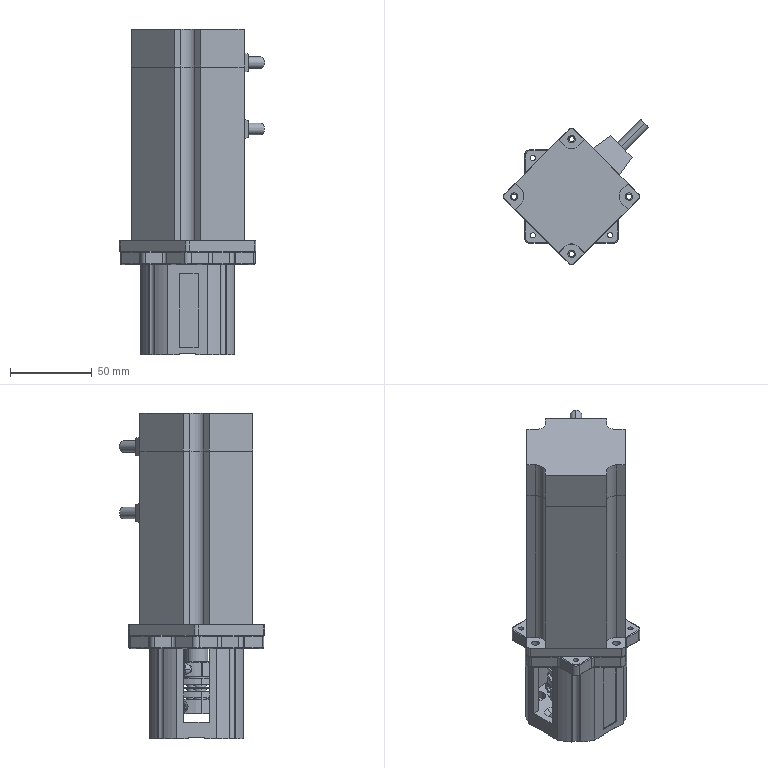Part | STEP file | Copy of 400W motor assembly (universal motor base)^K50A-1H20-S(formula driven)-L300-motor left- | 10 solids | 543 faces | box 88.621 x 88.621 x 198.5 mm | volume 512392 mm3 | cylinder 244 | plane 205 | cone 49 | torus 45 | commonest cylinder face diameters 1 x40 7 x36 6 x22 3.3 x21 8 x19 3.2 x16